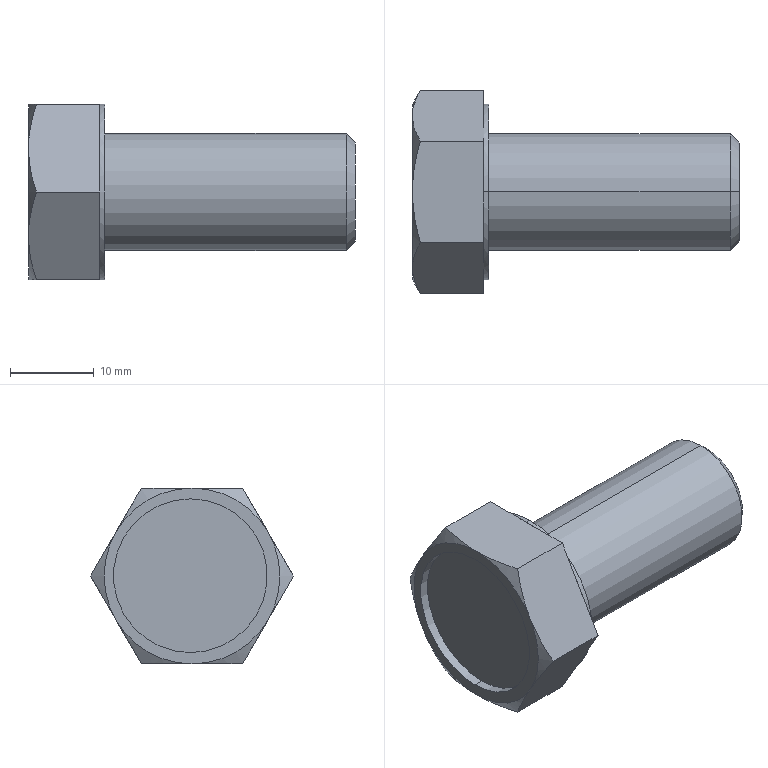Part | STEP file | formed hex screw_am_B18.2.3.2M - Formed hex screw, M14 x 2.0 x 30 --30WN | 1 solid | 30 faces | box 39.09 x 24.249 x 21 mm | volume 7732 mm3 | plane 16 | cone 8 | cylinder 6 | commonest cylinder face diameters 14 x2 18.375 x2 21 x2